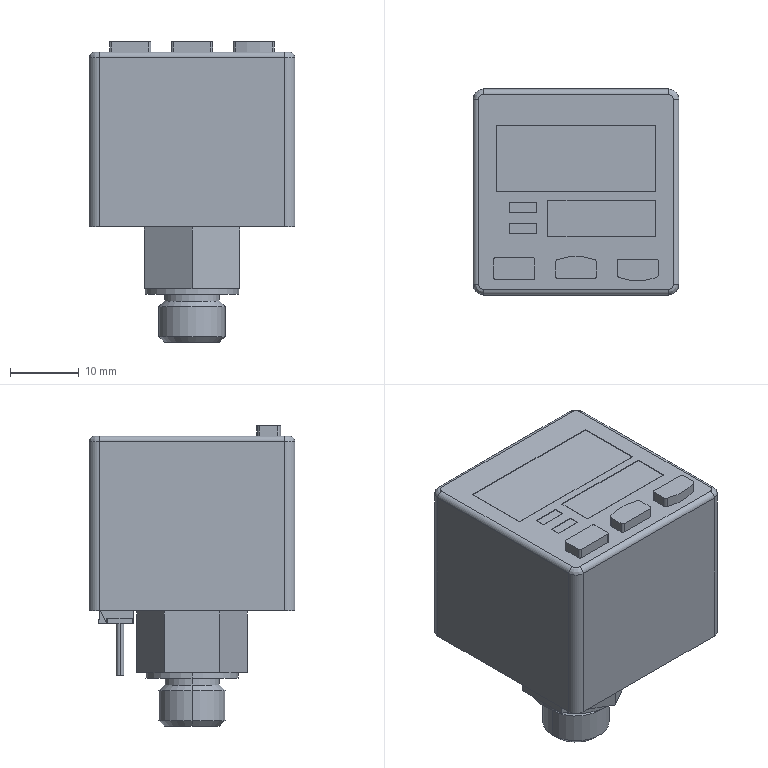Part | STEP file | DP101-E-P | 2 solids | 202 faces | box 30 x 30 x 43.8 mm | volume 24545 mm3 | plane 138 | cylinder 52 | cone 8 | spline 4 | commonest cylinder face diameters 0.6 x8 1.1 x8 3 x8 0.2 x4 1 x4 1.6 x4